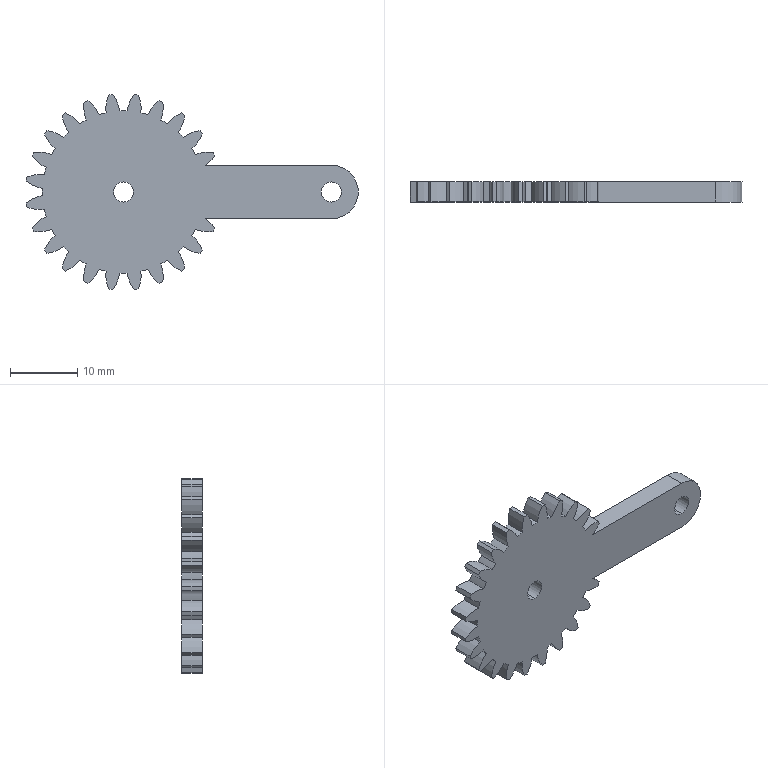Part | SolidWorks | features Extrusion 1 | 1 solid | 100 faces | box 49.537 x 3 x 29.075 mm | volume 2135 mm3 | cylinder 96 | plane 4 | commonest cylinder face diameters 10.8 x47 24.185 x22 29.25 x22 3 x4 8 x1